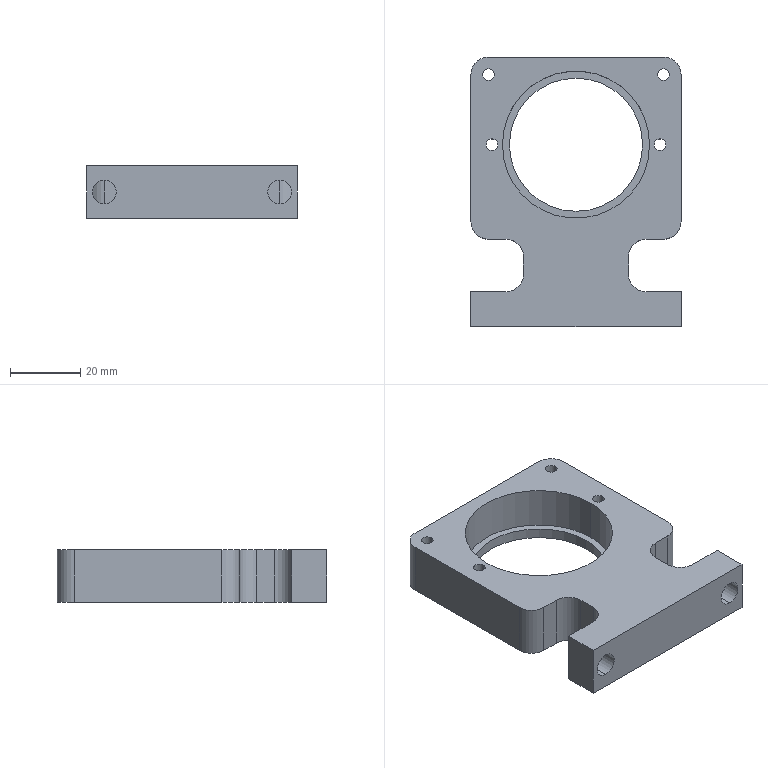Part | SolidWorks | features ICE 3, HoleWzd 2, Extrusion 1, Fillet 1 | 1 solid | 39 faces | box 60 x 77 x 15 mm | volume 41283 mm3 | cylinder 24 | plane 15 | commonest cylinder face diameters 3.3 x8 10 x8 6.8 x4 38 x2 42 x2
STEP:
#1=CARTESIAN_POINT('',(-26.65,72.,-7.5));
#2=VERTEX_POINT('',#1);
#3=CARTESIAN_POINT('',(-23.35,72.,-7.5));
#4=VERTEX_POINT('',#3);
#5=CARTESIAN_POINT('',(-25.,72.,-7.5));
#6=DIRECTION('',(0.,0.,1.));
#7=DIRECTION('',(1.,0.,0.));
#8=AXIS2_PLACEMENT_3D('',#5,#6,#7);
#9=CIRCLE('',#8,1.65);
#10=EDGE_CURVE('',#2,#4,#9,.T.);
#11=ORIENTED_EDGE('',*,*,#10,.F.);
#12=CARTESIAN_POINT('',(-26.65,72.,7.5));
#13=VERTEX_POINT('',#12);
#14=CARTESIAN_POINT('',(-26.65,72.,7.5));
#15=DIRECTION('',(0.,0.,1.));
#16=VECTOR('',#15,1000.);
#17=LINE('',#14,#16);
#18=EDGE_CURVE('',#2,#13,#17,.T.);
#19=ORIENTED_EDGE('',*,*,#18,.T.);
#20=CARTESIAN_POINT('',(-23.35,72.,7.5));
#21=VERTEX_POINT('',#20);
#22=CARTESIAN_POINT('',(-25.,72.,7.5));
#23=DIRECTION('',(0.,0.,1.));
#24=DIRECTION('',(1.,0.,0.));
#25=AXIS2_PLACEMENT_3D('',#22,#23,#24);
#26=CIRCLE('',#25,1.65);
#27=EDGE_CURVE('',#13,#21,#26,.T.);
#28=ORIENTED_EDGE('',*,*,#27,.T.);
#29=CARTESIAN_POINT('',(-23.35,72.,7.5));
#30=DIRECTION('',(0.,0.,1.));
#31=VECTOR('',#30,1000.);
#32=LINE('',#29,#31);
#33=EDGE_CURVE('',#4,#21,#32,.T.);
#34=ORIENTED_EDGE('',*,*,#33,.F.);
#35=EDGE_LOOP('',(#11,#19,#28,#34));
#36=FACE_OUTER_BOUND('',#35,.T.);
#37=CARTESIAN_POINT('',(-25.,72.,7.5));
#38=DIRECTION('',(0.,0.,1.));
#39=DIRECTION('',(1.,0.,0.));
#40=AXIS2_PLACEMENT_3D('',#37,#38,#39);
#41=CYLINDRICAL_SURFACE('',#40,1.65);
#42=ADVANCED_FACE('',(#36),#41,.F.);
#43=CARTESIAN_POINT('',(23.35,72.,-7.5));
#44=VERTEX_POINT('',#43);
#45=CARTESIAN_POINT('',(26.65,72.,-7.5));
#46=VERTEX_POINT('',#45);
#47=CARTESIAN_POINT('',(25.,72.,-7.5));
#48=DIRECTION('',(0.,0.,1.));
#49=DIRECTION('',(1.,0.,0.));
#50=AXIS2_PLACEMENT_3D('',#47,#48,#49);
#51=CIRCLE('',#50,1.65);
#52=EDGE_CURVE('',#44,#46,#51,.T.);
#53=ORIENTED_EDGE('',*,*,#52,.F.);
#54=CARTESIAN_POINT('',(23.35,72.,7.5));
#55=VERTEX_POINT('',#54);
#56=CARTESIAN_POINT('',(23.35,72.,7.5));
#57=DIRECTION('',(0.,0.,1.));
#58=VECTOR('',#57,1000.);
#59=LINE('',#56,#58);
#60=EDGE_CURVE('',#44,#55,#59,.T.);
#61=ORIENTED_EDGE('',*,*,#60,.T.);
#62=CARTESIAN_POINT('',(26.65,72.,7.5));
#63=VERTEX_POINT('',#62);
#64=CARTESIAN_POINT('',(25.,72.,7.5));
#65=DIRECTION('',(0.,0.,1.));
#66=DIRECTION('',(1.,0.,0.));
#67=AXIS2_PLACEMENT_3D('',#64,#65,#66);
#68=CIRCLE('',#67,1.65);
#69=EDGE_CURVE('',#55,#63,#68,.T.);
#70=ORIENTED_EDGE('',*,*,#69,.T.);
#71=CARTESIAN_POINT('',(26.65,72.,7.5));
#72=DIRECTION('',(0.,0.,1.));
#73=VECTOR('',#72,1000.);
#74=LINE('',#71,#73);
#75=EDGE_CURVE('',#46,#63,#74,.T.);
#76=ORIENTED_EDGE('',*,*,#75,.F.);
#77=EDGE_LOOP('',(#53,#61,#70,#76));
#78=FACE_OUTER_BOUND('',#77,.T.);
#79=CARTESIAN_POINT('',(25.,72.,7.5));
#80=DIRECTION('',(0.,0.,1.));
#81=DIRECTION('',(1.,0.,0.));
#82=AXIS2_PLACEMENT_3D('',#79,#80,#81);
#83=CYLINDRICAL_SURFACE('',#82,1.65);
#84=ADVANCED_FACE('',(#78),#83,.F.);
#85=CARTESIAN_POINT('',(22.35,52.,-7.5));
#86=VERTEX_POINT('',#85);
#87=CARTESIAN_POINT('',(25.65,52.,-7.5));
#88=VERTEX_POINT('',#87);
#89=CARTESIAN_POINT('',(24.,52.,-7.5));
#90=DIRECTION('',(0.,0.,1.));
#91=DIRECTION('',(1.,0.,0.));
#92=AXIS2_PLACEMENT_3D('',#89,#90,#91);
#93=CIRCLE('',#92,1.65);
#94=EDGE_CURVE('',#86,#88,#93,.T.);
#95=ORIENTED_EDGE('',*,*,#94,.F.);
#96=CARTESIAN_POINT('',(22.35,52.,7.5));
#97=VERTEX_POINT('',#96);
#98=CARTESIAN_POINT('',(22.35,52.,7.5));
#99=DIRECTION('',(0.,0.,1.));
#100=VECTOR('',#99,1000.);
#101=LINE('',#98,#100);
#102=EDGE_CURVE('',#86,#97,#101,.T.);
#103=ORIENTED_EDGE('',*,*,#102,.T.);
#104=CARTESIAN_POINT('',(25.65,52.,7.5));
#105=VERTEX_POINT('',#104);
#106=CARTESIAN_POINT('',(24.,52.,7.5));
#107=DIRECTION('',(0.,0.,1.));
#108=DIRECTION('',(1.,0.,0.));
#109=AXIS2_PLACEMENT_3D('',#106,#107,#108);
#110=CIRCLE('',#109,1.65);
#111=EDGE_CURVE('',#97,#105,#110,.T.);
#112=ORIENTED_EDGE('',*,*,#111,.T.);
#113=CARTESIAN_POINT('',(25.65,52.,7.5));
#114=DIRECTION('',(0.,0.,1.));
#115=VECTOR('',#114,1000.);
#116=LINE('',#113,#115);
#117=EDGE_CURVE('',#88,#105,#116,.T.);
#118=ORIENTED_EDGE('',*,*,#117,.F.);
#119=EDGE_LOOP('',(#95,#103,#112,#118));
#120=FACE_OUTER_BOUND('',#119,.T.);
#121=CARTESIAN_POINT('',(24.,52.,7.5));
#122=DIRECTION('',(0.,0.,1.));
#123=DIRECTION('',(1.,0.,0.));
#124=AXIS2_PLACEMENT_3D('',#121,#122,#123);
#125=CYLINDRICAL_SURFACE('',#124,1.65);
#126=ADVANCED_FACE('',(#120),#125,.F.);
#127=CARTESIAN_POINT('',(-25.65,52.,-7.5));
#128=VERTEX_POINT('',#127);
#129=CARTESIAN_POINT('',(-22.35,52.,-7.5));
#130=VERTEX_POINT('',#129);
#131=CARTESIAN_POINT('',(-24.,52.,-7.5));
#132=DIRECTION('',(0.,0.,1.));
#133=DIRECTION('',(1.,0.,0.));
#134=AXIS2_PLACEMENT_3D('',#131,#132,#133);
#135=CIRCLE('',#134,1.65);
#136=EDGE_CURVE('',#128,#130,#135,.T.);
#137=ORIENTED_EDGE('',*,*,#136,.F.);
#138=CARTESIAN_POINT('',(-25.65,52.,7.5));
#139=VERTEX_POINT('',#138);
#140=CARTESIAN_POINT('',(-25.65,52.,7.5));
#141=DIRECTION('',(0.,0.,1.));
#142=VECTOR('',#141,1000.);
#143=LINE('',#140,#142);
#144=EDGE_CURVE('',#128,#139,#143,.T.);
#145=ORIENTED_EDGE('',*,*,#144,.T.);
#146=CARTESIAN_POINT('',(-22.35,52.,7.5));
#147=VERTEX_POINT('',#146);
#148=CARTESIAN_POINT('',(-24.,52.,7.5));
#149=DIRECTION('',(0.,0.,1.));
#150=DIRECTION('',(1.,0.,0.));
#151=AXIS2_PLACEMENT_3D('',#148,#149,#150);
#152=CIRCLE('',#151,1.65);
#153=EDGE_CURVE('',#139,#147,#152,.T.);
#154=ORIENTED_EDGE('',*,*,#153,.T.);
#155=CARTESIAN_POINT('',(-22.35,52.,7.5));
#156=DIRECTION('',(0.,0.,1.));
#157=VECTOR('',#156,1000.);
#158=LINE('',#155,#157);
#159=EDGE_CURVE('',#130,#147,#158,.T.);
#160=ORIENTED_EDGE('',*,*,#159,.F.);
#161=EDGE_LOOP('',(#137,#145,#154,#160));
#162=FACE_OUTER_BOUND('',#161,.T.);
#163=CARTESIAN_POINT('',(-24.,52.,7.5));
#164=DIRECTION('',(0.,0.,1.));
#165=DIRECTION('',(1.,0.,0.));
#166=AXIS2_PLACEMENT_3D('',#163,#164,#165);
#167=CYLINDRICAL_SURFACE('',#166,1.65);
#168=ADVANCED_FACE('',(#162),#167,.F.);
#169=CARTESIAN_POINT('',(-21.,52.,-4.5));
#170=VERTEX_POINT('',#169);
#171=CARTESIAN_POINT('',(21.,52.,-4.5));
#172=VERTEX_POINT('',#171);
#173=CARTESIAN_POINT('',(0.,52.,-4.5));
#174=DIRECTION('',(0.,0.,1.));
#175=DIRECTION('',(1.,0.,0.));
#176=AXIS2_PLACEMENT_3D('',#173,#174,#175);
#177=CIRCLE('',#176,21.);
#178=EDGE_CURVE('',#170,#172,#177,.T.);
#179=ORIENTED_EDGE('',*,*,#178,.F.);
#180=CARTESIAN_POINT('',(-21.,52.,7.5));
#181=VERTEX_POINT('',#180);
#182=CARTESIAN_POINT('',(-21.,52.,-4.5));
#183=DIRECTION('',(0.,0.,1.));
#184=VECTOR('',#183,1000.);
#185=LINE('',#182,#184);
#186=EDGE_CURVE('',#170,#181,#185,.T.);
#187=ORIENTED_EDGE('',*,*,#186,.T.);
#188=CARTESIAN_POINT('',(21.,52.,7.5));
#189=VERTEX_POINT('',#188);
#190=CARTESIAN_POINT('',(0.,52.,7.5));
#191=DIRECTION('',(0.,0.,1.));
#192=DIRECTION('',(1.,0.,0.));
#193=AXIS2_PLACEMENT_3D('',#190,#191,#192);
#194=CIRCLE('',#193,21.);
#195=EDGE_CURVE('',#181,#189,#194,.T.);
#196=ORIENTED_EDGE('',*,*,#195,.T.);
#197=CARTESIAN_POINT('',(21.,52.,-4.5));
#198=DIRECTION('',(0.,0.,1.));
#199=VECTOR('',#198,1000.);
#200=LINE('',#197,#199);
#201=EDGE_CURVE('',#172,#189,#200,.T.);
#202=ORIENTED_EDGE('',*,*,#201,.F.);
#203=EDGE_LOOP('',(#179,#187,#196,#202));
#204=FACE_OUTER_BOUND('',#203,.T.);
#205=CARTESIAN_POINT('',(0.,52.,-4.5));
#206=DIRECTION('',(0.,0.,1.));
#207=DIRECTION('',(1.,0.,0.));
#208=AXIS2_PLACEMENT_3D('',#205,#206,#207);
#209=CYLINDRICAL_SURFACE('',#208,21.);
#210=ADVANCED_FACE('',(#204),#209,.F.);
#211=CARTESIAN_POINT('',(-25.,10.,3.4));
#212=VERTEX_POINT('',#211);
#213=CARTESIAN_POINT('',(-25.,10.,-3.4));
#214=VERTEX_POINT('',#213);
#215=CARTESIAN_POINT('',(-25.,10.,0.));
#216=DIRECTION('',(0.,-1.,0.));
#217=DIRECTION('',(0.,0.,-1.));
#218=AXIS2_PLACEMENT_3D('',#215,#216,#217);
#219=CIRCLE('',#218,3.4);
#220=EDGE_CURVE('',#212,#214,#219,.T.);
#221=ORIENTED_EDGE('',*,*,#220,.F.);
#222=CARTESIAN_POINT('',(-25.,0.,3.4));
#223=VERTEX_POINT('',#222);
#224=CARTESIAN_POINT('',(-25.,15.,3.4));
#225=DIRECTION('',(0.,-1.,0.));
#226=VECTOR('',#225,1000.);
#227=LINE('',#224,#226);
#228=EDGE_CURVE('',#212,#223,#227,.T.);
#229=ORIENTED_EDGE('',*,*,#228,.T.);
#230=CARTESIAN_POINT('',(-25.,0.,-3.4));
#231=VERTEX_POINT('',#230);
#232=CARTESIAN_POINT('',(-25.,0.,0.));
#233=DIRECTION('',(0.,-1.,0.));
#234=DIRECTION('',(0.,0.,-1.));
#235=AXIS2_PLACEMENT_3D('',#232,#233,#234);
#236=CIRCLE('',#235,3.4);
#237=EDGE_CURVE('',#223,#231,#236,.T.);
#238=ORIENTED_EDGE('',*,*,#237,.T.);
#239=CARTESIAN_POINT('',(-25.,15.,-3.4));
#240=DIRECTION('',(0.,-1.,0.));
#241=VECTOR('',#240,1000.);
#242=LINE('',#239,#241);
#243=EDGE_CURVE('',#214,#231,#242,.T.);
#244=ORIENTED_EDGE('',*,*,#243,.F.);
#245=EDGE_LOOP('',(#221,#229,#238,#244));
#246=FACE_OUTER_BOUND('',#245,.T.);
#247=CARTESIAN_POINT('',(-25.,15.,0.));
#248=DIRECTION('',(0.,-1.,0.));
#249=DIRECTION('',(0.,0.,-1.));
#250=AXIS2_PLACEMENT_3D('',#247,#248,#249);
#251=CYLINDRICAL_SURFACE('',#250,3.4);
#252=ADVANCED_FACE('',(#246),#251,.F.);
#253=CARTESIAN_POINT('',(25.,10.,3.4));
#254=VERTEX_POINT('',#253);
#255=CARTESIAN_POINT('',(25.,10.,-3.4));
#256=VERTEX_POINT('',#255);
#257=CARTESIAN_POINT('',(25.,10.,0.));
#258=DIRECTION('',(0.,-1.,0.));
#259=DIRECTION('',(0.,0.,-1.));
#260=AXIS2_PLACEMENT_3D('',#257,#258,#259);
#261=CIRCLE('',#260,3.4);
#262=EDGE_CURVE('',#254,#256,#261,.T.);
#263=ORIENTED_EDGE('',*,*,#262,.F.);
#264=CARTESIAN_POINT('',(25.,0.,3.4));
#265=VERTEX_POINT('',#264);
#266=CARTESIAN_POINT('',(25.,15.,3.4));
#267=DIRECTION('',(0.,-1.,0.));
#268=VECTOR('',#267,1000.);
#269=LINE('',#266,#268);
#270=EDGE_CURVE('',#254,#265,#269,.T.);
#271=ORIENTED_EDGE('',*,*,#270,.T.);
#272=CARTESIAN_POINT('',(25.,0.,-3.4));
#273=VERTEX_POINT('',#272);
#274=CARTESIAN_POINT('',(25.,0.,0.));
#275=DIRECTION('',(0.,-1.,0.));
#276=DIRECTION('',(0.,0.,1.));
#277=AXIS2_PLACEMENT_3D('',#274,#275,#276);
#278=CIRCLE('',#277,3.4);
#279=EDGE_CURVE('',#265,#273,#278,.T.);
#280=ORIENTED_EDGE('',*,*,#279,.T.);
#281=CARTESIAN_POINT('',(25.,15.,-3.4));
#282=DIRECTION('',(0.,-1.,0.));
#283=VECTOR('',#282,1000.);
#284=LINE('',#281,#283);
#285=EDGE_CURVE('',#256,#273,#284,.T.);
#286=ORIENTED_EDGE('',*,*,#285,.F.);
#287=EDGE_LOOP('',(#263,#271,#280,#286));
#288=FACE_OUTER_BOUND('',#287,.T.);
#289=CARTESIAN_POINT('',(25.,15.,0.));
#290=DIRECTION('',(0.,-1.,0.));
#291=DIRECTION('',(0.,0.,-1.));
#292=AXIS2_PLACEMENT_3D('',#289,#290,#291);
#293=CYLINDRICAL_SURFACE('',#292,3.4);
#294=ADVANCED_FACE('',(#288),#293,.F.);
#295=CARTESIAN_POINT('',(-19.,52.,-7.5));
#296=VERTEX_POINT('',#295);
#297=CARTESIAN_POINT('',(19.,52.,-7.5));
#298=VERTEX_POINT('',#297);
#299=CARTESIAN_POINT('',(0.,52.,-7.5));
#300=DIRECTION('',(0.,0.,1.));
#301=DIRECTION('',(1.,0.,0.));
#302=AXIS2_PLACEMENT_3D('',#299,#300,#301);
#303=CIRCLE('',#302,19.);
#304=EDGE_CURVE('',#296,#298,#303,.T.);
#305=ORIENTED_EDGE('',*,*,#304,.F.);
#306=CARTESIAN_POINT('',(-19.,52.,-4.5));
#307=VERTEX_POINT('',#306);
#308=CARTESIAN_POINT('',(-19.,52.,-7.5));
#309=DIRECTION('',(0.,0.,1.));
#310=VECTOR('',#309,1000.);
#311=LINE('',#308,#310);
#312=EDGE_CURVE('',#296,#307,#311,.T.);
#313=ORIENTED_EDGE('',*,*,#312,.T.);
#314=CARTESIAN_POINT('',(19.,52.,-4.5));
#315=VERTEX_POINT('',#314);
#316=CARTESIAN_POINT('',(0.,52.,-4.5));
#317=DIRECTION('',(0.,0.,-1.));
#318=DIRECTION('',(1.,0.,0.));
#319=AXIS2_PLACEMENT_3D('',#316,#317,#318);
#320=CIRCLE('',#319,19.);
#321=EDGE_CURVE('',#315,#307,#320,.T.);
#322=ORIENTED_EDGE('',*,*,#321,.F.);
#323=CARTESIAN_POINT('',(19.,52.,-7.5));
#324=DIRECTION('',(0.,0.,1.));
#325=VECTOR('',#324,1000.);
#326=LINE('',#323,#325);
#327=EDGE_CURVE('',#298,#315,#326,.T.);
#328=ORIENTED_EDGE('',*,*,#327,.F.);
#329=EDGE_LOOP('',(#305,#313,#322,#328));
#330=FACE_OUTER_BOUND('',#329,.T.);
#331=CARTESIAN_POINT('',(0.,52.,-7.5));
#332=DIRECTION('',(0.,0.,1.));
#333=DIRECTION('',(1.,0.,0.));
#334=AXIS2_PLACEMENT_3D('',#331,#332,#333);
#335=CYLINDRICAL_SURFACE('',#334,19.);
#336=ADVANCED_FACE('',(#330),#335,.F.);
#337=ORIENTED_EDGE('',*,*,#312,.F.);
#338=CARTESIAN_POINT('',(0.,52.,-7.5));
#339=DIRECTION('',(0.,0.,1.));
#340=DIRECTION('',(1.,0.,0.));
#341=AXIS2_PLACEMENT_3D('',#338,#339,#340);
#342=CIRCLE('',#341,19.);
#343=EDGE_CURVE('',#298,#296,#342,.T.);
#344=ORIENTED_EDGE('',*,*,#343,.F.);
#345=ORIENTED_EDGE('',*,*,#327,.T.);
#346=CARTESIAN_POINT('',(0.,52.,-4.5));
#347=DIRECTION('',(0.,0.,-1.));
#348=DIRECTION('',(1.,0.,0.));
#349=AXIS2_PLACEMENT_3D('',#346,#347,#348);
#350=CIRCLE('',#349,19.);
#351=EDGE_CURVE('',#307,#315,#350,.T.);
#352=ORIENTED_EDGE('',*,*,#351,.F.);
#353=EDGE_LOOP('',(#337,#344,#345,#352));
#354=FACE_OUTER_BOUND('',#353,.T.);
#355=CARTESIAN_POINT('',(0.,52.,-7.5));
#356=DIRECTION('',(0.,0.,1.));
#357=DIRECTION('',(1.,0.,0.));
#358=AXIS2_PLACEMENT_3D('',#355,#356,#357);
#359=CYLINDRICAL_SURFACE('',#358,19.);
#360=ADVANCED_FACE('',(#354),#359,.F.);
#361=CARTESIAN_POINT('',(-25.,25.,7.5));
#362=VERTEX_POINT('',#361);
#363=CARTESIAN_POINT('',(-20.,25.,7.5));
#364=VERTEX_POINT('',#363);
#365=CARTESIAN_POINT('',(-15.,25.,7.5));
#366=DIRECTION('',(1.,0.,0.));
#367=VECTOR('',#366,1000.);
#368=LINE('',#365,#367);
#369=EDGE_CURVE('',#362,#364,#368,.T.);
#370=ORIENTED_EDGE('',*,*,#369,.F.);
#371=CARTESIAN_POINT('',(-25.,25.,-7.5));
#372=VERTEX_POINT('',#371);
#373=CARTESIAN_POINT('',(-25.,25.,7.5));
#374=DIRECTION('',(0.,0.,-1.));
#375=VECTOR('',#374,1000.);
#376=LINE('',#373,#375);
#377=EDGE_CURVE('',#362,#372,#376,.T.);
#378=ORIENTED_EDGE('',*,*,#377,.T.);
#379=CARTESIAN_POINT('',(-20.,25.,-7.5));
#380=VERTEX_POINT('',#379);
#381=CARTESIAN_POINT('',(-15.,25.,-7.5));
#382=DIRECTION('',(1.,0.,0.));
#383=VECTOR('',#382,1000.);
#384=LINE('',#381,#383);
#385=EDGE_CURVE('',#372,#380,#384,.T.);
#386=ORIENTED_EDGE('',*,*,#385,.T.);
#387=CARTESIAN_POINT('',(-20.,25.,7.5));
#388=DIRECTION('',(0.,0.,1.));
#389=VECTOR('',#388,1000.);
#390=LINE('',#387,#389);
#391=EDGE_CURVE('',#380,#364,#390,.T.);
#392=ORIENTED_EDGE('',*,*,#391,.T.);
#393=EDGE_LOOP('',(#370,#378,#386,#392));
#394=FACE_OUTER_BOUND('',#393,.T.);
#395=CARTESIAN_POINT('',(-15.,25.,7.5));
#396=DIRECTION('',(0.,1.,0.));
#397=DIRECTION('',(-1.,0.,0.));
#398=AXIS2_PLACEMENT_3D('',#395,#396,#397);
#399=PLANE('',#398);
#400=ADVANCED_FACE('',(#394),#399,.F.);
#401=CARTESIAN_POINT('',(-15.,20.,-7.5));
#402=VERTEX_POINT('',#401);
#403=CARTESIAN_POINT('',(-15.,15.,-7.5));
#404=VERTEX_POINT('',#403);
#405=CARTESIAN_POINT('',(-15.,10.,-7.5));
#406=DIRECTION('',(0.,-1.,0.));
#407=VECTOR('',#406,1000.);
#408=LINE('',#405,#407);
#409=EDGE_CURVE('',#402,#404,#408,.T.);
#410=ORIENTED_EDGE('',*,*,#409,.T.);
#411=CARTESIAN_POINT('',(-15.,15.,7.5));
#412=VERTEX_POINT('',#411);
#413=CARTESIAN_POINT('',(-15.,15.,7.5));
#414=DIRECTION('',(0.,0.,1.));
#415=VECTOR('',#414,1000.);
#416=LINE('',#413,#415);
#417=EDGE_CURVE('',#404,#412,#416,.T.);
#418=ORIENTED_EDGE('',*,*,#417,.T.);
#419=CARTESIAN_POINT('',(-15.,20.,7.5));
#420=VERTEX_POINT('',#419);
#421=CARTESIAN_POINT('',(-15.,10.,7.5));
#422=DIRECTION('',(0.,-1.,0.));
#423=VECTOR('',#422,1000.);
#424=LINE('',#421,#423);
#425=EDGE_CURVE('',#420,#412,#424,.T.);
#426=ORIENTED_EDGE('',*,*,#425,.F.);
#427=CARTESIAN_POINT('',(-15.,20.,-7.5));
#428=DIRECTION('',(0.,0.,-1.));
#429=VECTOR('',#428,1000.);
#430=LINE('',#427,#429);
#431=EDGE_CURVE('',#420,#402,#430,.T.);
#432=ORIENTED_EDGE('',*,*,#431,.T.);
#433=EDGE_LOOP('',(#410,#418,#426,#432));
#434=FACE_OUTER_BOUND('',#433,.T.);
#435=CARTESIAN_POINT('',(-15.,10.,7.5));
#436=DIRECTION('',(1.,0.,0.));
#437=DIRECTION('',(0.,1.,0.));
#438=AXIS2_PLACEMENT_3D('',#435,#436,#437);
#439=PLANE('',#438);
#440=ADVANCED_FACE('',(#434),#439,.F.);
#441=CARTESIAN_POINT('',(-25.,10.,0.));
#442=DIRECTION('',(0.,-1.,0.));
#443=DIRECTION('',(0.,0.,-1.));
#444=AXIS2_PLACEMENT_3D('',#441,#442,#443);
#445=CIRCLE('',#444,3.4);
#446=EDGE_CURVE('',#214,#212,#445,.T.);
#447=ORIENTED_EDGE('',*,*,#446,.T.);
#448=ORIENTED_EDGE('',*,*,#220,.T.);
#449=EDGE_LOOP('',(#447,#448));
#450=FACE_BOUND('',#449,.T.);
#451=CARTESIAN_POINT('',(-20.,10.,7.5));
#452=VERTEX_POINT('',#451);
#453=CARTESIAN_POINT('',(-30.,10.,7.5));
#454=VERTEX_POINT('',#453);
#455=CARTESIAN_POINT('',(-30.,10.,7.5));
#456=DIRECTION('',(-1.,0.,0.));
#457=VECTOR('',#456,1000.);
#458=LINE('',#455,#457);
#459=EDGE_CURVE('',#452,#454,#458,.T.);
#460=ORIENTED_EDGE('',*,*,#459,.F.);
#461=CARTESIAN_POINT('',(-20.,10.,-7.5));
#462=VERTEX_POINT('',#461);
#463=CARTESIAN_POINT('',(-20.,10.,-7.5));
#464=DIRECTION('',(0.,0.,-1.));
#465=VECTOR('',#464,1000.);
#466=LINE('',#463,#465);
#467=EDGE_CURVE('',#452,#462,#466,.T.);
#468=ORIENTED_EDGE('',*,*,#467,.T.);
#469=CARTESIAN_POINT('',(-30.,10.,-7.5));
#470=VERTEX_POINT('',#469);
#471=CARTESIAN_POINT('',(-30.,10.,-7.5));
#472=DIRECTION('',(-1.,0.,0.));
#473=VECTOR('',#472,1000.);
#474=LINE('',#471,#473);
#475=EDGE_CURVE('',#462,#470,#474,.T.);
#476=ORIENTED_EDGE('',*,*,#475,.T.);
#477=CARTESIAN_POINT('',(-30.,10.,7.5));
#478=DIRECTION('',(0.,0.,-1.));
#479=VECTOR('',#478,1000.);
#480=LINE('',#477,#479);
#481=EDGE_CURVE('',#454,#470,#480,.T.);
#482=ORIENTED_EDGE('',*,*,#481,.F.);
#483=EDGE_LOOP('',(#460,#468,#476,#482));
#484=FACE_OUTER_BOUND('',#483,.T.);
#485=CARTESIAN_POINT('',(-30.,10.,7.5));
#486=DIRECTION('',(0.,-1.,0.));
#487=DIRECTION('',(0.,0.,-1.));
#488=AXIS2_PLACEMENT_3D('',#485,#486,#487);
#489=PLANE('',#488);
#490=ADVANCED_FACE('',(#450,#484),#489,.F.);
#491=CARTESIAN_POINT('',(-30.,0.,-7.5));
#492=VERTEX_POINT('',#491);
#493=CARTESIAN_POINT('',(-30.,0.,-7.5));
#494=DIRECTION('',(0.,-1.,0.));
#495=VECTOR('',#494,1000.);
#496=LINE('',#493,#495);
#497=EDGE_CURVE('',#470,#492,#496,.T.);
#498=ORIENTED_EDGE('',*,*,#497,.T.);
#499=CARTESIAN_POINT('',(-30.,0.,7.5));
#500=VERTEX_POINT('',#499);
#501=CARTESIAN_POINT('',(-30.,0.,7.5));
#502=DIRECTION('',(0.,0.,-1.));
#503=VECTOR('',#502,1000.);
#504=LINE('',#501,#503);
#505=EDGE_CURVE('',#500,#492,#504,.T.);
#506=ORIENTED_EDGE('',*,*,#505,.F.);
#507=CARTESIAN_POINT('',(-30.,0.,7.5));
#508=DIRECTION('',(0.,-1.,0.));
#509=VECTOR('',#508,1000.);
#510=LINE('',#507,#509);
#511=EDGE_CURVE('',#454,#500,#510,.T.);
#512=ORIENTED_EDGE('',*,*,#511,.F.);
#513=ORIENTED_EDGE('',*,*,#481,.T.);
#514=EDGE_LOOP('',(#498,#506,#512,#513));
#515=FACE_OUTER_BOUND('',#514,.T.);
#516=CARTESIAN_POINT('',(-30.,0.,7.5));
#517=DIRECTION('',(1.,0.,0.));
#518=DIRECTION('',(0.,0.,-1.));
#519=AXIS2_PLACEMENT_3D('',#516,#517,#518);
#520=PLANE('',#519);
#521=ADVANCED_FACE('',(#515),#520,.F.);
#522=CARTESIAN_POINT('',(-25.,0.,0.));
#523=DIRECTION('',(0.,-1.,0.));
#524=DIRECTION('',(0.,0.,-1.));
#525=AXIS2_PLACEMENT_3D('',#522,#523,#524);
#526=CIRCLE('',#525,3.4);
#527=EDGE_CURVE('',#231,#223,#526,.T.);
#528=ORIENTED_EDGE('',*,*,#527,.F.);
#529=ORIENTED_EDGE('',*,*,#237,.F.);
#530=EDGE_LOOP('',(#528,#529));
#531=FACE_BOUND('',#530,.T.);
#532=CARTESIAN_POINT('',(25.,0.,0.));
#533=DIRECTION('',(0.,-1.,0.));
#534=DIRECTION('',(0.,0.,1.));
#535=AXIS2_PLACEMENT_3D('',#532,#533,#534);
#536=CIRCLE('',#535,3.4);
#537=EDGE_CURVE('',#273,#265,#536,.T.);
#538=ORIENTED_EDGE('',*,*,#537,.F.);
#539=ORIENTED_EDGE('',*,*,#279,.F.);
#540=EDGE_LOOP('',(#538,#539));
#541=FACE_BOUND('',#540,.T.);
#542=CARTESIAN_POINT('',(30.,0.,-7.5));
#543=VERTEX_POINT('',#542);
#544=CARTESIAN_POINT('',(30.,0.,-7.5));
#545=DIRECTION('',(1.,0.,0.));
#546=VECTOR('',#545,1000.);
#547=LINE('',#544,#546);
#548=EDGE_CURVE('',#492,#543,#547,.T.);
#549=ORIENTED_EDGE('',*,*,#548,.T.);
#550=CARTESIAN_POINT('',(30.,0.,7.5));
#551=VERTEX_POINT('',#550);
#552=CARTESIAN_POINT('',(30.,0.,7.5));
#553=DIRECTION('',(0.,0.,-1.));
#554=VECTOR('',#553,1000.);
#555=LINE('',#552,#554);
#556=EDGE_CURVE('',#551,#543,#555,.T.);
#557=ORIENTED_EDGE('',*,*,#556,.F.);
#558=CARTESIAN_POINT('',(30.,0.,7.5));
#559=DIRECTION('',(1.,0.,0.));
#560=VECTOR('',#559,1000.);
#561=LINE('',#558,#560);
#562=EDGE_CURVE('',#500,#551,#561,.T.);
#563=ORIENTED_EDGE('',*,*,#562,.F.);
#564=ORIENTED_EDGE('',*,*,#505,.T.);
#565=EDGE_LOOP('',(#549,#557,#563,#564));
#566=FACE_OUTER_BOUND('',#565,.T.);
#567=CARTESIAN_POINT('',(30.,0.,7.5));
#568=DIRECTION('',(0.,1.,0.));
#569=DIRECTION('',(0.,0.,1.));
#570=AXIS2_PLACEMENT_3D('',#567,#568,#569);
#571=PLANE('',#570);
#572=ADVANCED_FACE('',(#531,#541,#566),#571,.F.);
#573=CARTESIAN_POINT('',(30.,10.,-7.5));
#574=VERTEX_POINT('',#573);
#575=CARTESIAN_POINT('',(30.,0.,-7.5));
#576=DIRECTION('',(0.,1.,0.));
#577=VECTOR('',#576,1000.);
#578=LINE('',#575,#577);
#579=EDGE_CURVE('',#543,#574,#578,.T.);
#580=ORIENTED_EDGE('',*,*,#579,.T.);
#581=CARTESIAN_POINT('',(30.,10.,7.5));
#582=VERTEX_POINT('',#581);
#583=CARTESIAN_POINT('',(30.,10.,7.5));
#584=DIRECTION('',(0.,0.,-1.));
#585=VECTOR('',#584,1000.);
#586=LINE('',#583,#585);
#587=EDGE_CURVE('',#582,#574,#586,.T.);
#588=ORIENTED_EDGE('',*,*,#587,.F.);
#589=CARTESIAN_POINT('',(30.,0.,7.5));
#590=DIRECTION('',(0.,1.,0.));
#591=VECTOR('',#590,1000.);
#592=LINE('',#589,#591);
#593=EDGE_CURVE('',#551,#582,#592,.T.);
#594=ORIENTED_EDGE('',*,*,#593,.F.);
#595=ORIENTED_EDGE('',*,*,#556,.T.);
#596=EDGE_LOOP('',(#580,#588,#594,#595));
#597=FACE_OUTER_BOUND('',#596,.T.);
#598=CARTESIAN_POINT('',(30.,0.,7.5));
#599=DIRECTION('',(-1.,0.,0.));
#600=DIRECTION('',(0.,0.,1.));
#601=AXIS2_PLACEMENT_3D('',#598,#599,#600);
#602=PLANE('',#601);
#603=ADVANCED_FACE('',(#597),#602,.F.);
#604=CARTESIAN_POINT('',(25.,10.,0.));
#605=DIRECTION('',(0.,-1.,0.));
#606=DIRECTION('',(0.,0.,-1.));
#607=AXIS2_PLACEMENT_3D('',#604,#605,#606);
#608=CIRCLE('',#607,3.4);
#609=EDGE_CURVE('',#256,#254,#608,.T.);
#610=ORIENTED_EDGE('',*,*,#609,.T.);
#611=ORIENTED_EDGE('',*,*,#262,.T.);
#612=EDGE_LOOP('',(#610,#611));
#613=FACE_BOUND('',#612,.T.);
#614=CARTESIAN_POINT('',(20.,10.,-7.5));
#615=VERTEX_POINT('',#614);
#616=CARTESIAN_POINT('',(30.,10.,-7.5));
#617=DIRECTION('',(-1.,0.,0.));
#618=VECTOR('',#617,1000.);
#619=LINE('',#616,#618);
#620=EDGE_CURVE('',#574,#615,#619,.T.);
#621=ORIENTED_EDGE('',*,*,#620,.T.);
#622=CARTESIAN_POINT('',(20.,10.,7.5));
#623=VERTEX_POINT('',#622);
#624=CARTESIAN_POINT('',(20.,10.,7.5));
#625=DIRECTION('',(0.,0.,1.));
#626=VECTOR('',#625,1000.);
#627=LINE('',#624,#626);
#628=EDGE_CURVE('',#615,#623,#627,.T.);
#629=ORIENTED_EDGE('',*,*,#628,.T.);
#630=CARTESIAN_POINT('',(30.,10.,7.5));
#631=DIRECTION('',(-1.,0.,0.));
#632=VECTOR('',#631,1000.);
#633=LINE('',#630,#632);
#634=EDGE_CURVE('',#582,#623,#633,.T.);
#635=ORIENTED_EDGE('',*,*,#634,.F.);
#636=ORIENTED_EDGE('',*,*,#587,.T.);
#637=EDGE_LOOP('',(#621,#629,#635,#636));
#638=FACE_OUTER_BOUND('',#637,.T.);
#639=CARTESIAN_POINT('',(30.,10.,7.5));
#640=DIRECTION('',(0.,-1.,0.));
#641=DIRECTION('',(0.,0.,-1.));
#642=AXIS2_PLACEMENT_3D('',#639,#640,#641);
#643=PLANE('',#642);
#644=ADVANCED_FACE('',(#613,#638),#643,.F.);
#645=CARTESIAN_POINT('',(15.,15.,-7.5));
#646=VERTEX_POINT('',#645);
#647=CARTESIAN_POINT('',(15.,20.,-7.5));
#648=VERTEX_POINT('',#647);
#649=CARTESIAN_POINT('',(15.,10.,-7.5));
#650=DIRECTION('',(0.,1.,0.));
#651=VECTOR('',#650,1000.);
#652=LINE('',#649,#651);
#653=EDGE_CURVE('',#646,#648,#652,.T.);
#654=ORIENTED_EDGE('',*,*,#653,.T.);
#655=CARTESIAN_POINT('',(15.,20.,7.5));
#656=VERTEX_POINT('',#655);
#657=CARTESIAN_POINT('',(15.,20.,7.5));
#658=DIRECTION('',(0.,0.,1.));
#659=VECTOR('',#658,1000.);
#660=LINE('',#657,#659);
#661=EDGE_CURVE('',#648,#656,#660,.T.);
#662=ORIENTED_EDGE('',*,*,#661,.T.);
#663=CARTESIAN_POINT('',(15.,15.,7.5));
#664=VERTEX_POINT('',#663);
#665=CARTESIAN_POINT('',(15.,10.,7.5));
#666=DIRECTION('',(0.,1.,0.));
#667=VECTOR('',#666,1000.);
#668=LINE('',#665,#667);
#669=EDGE_CURVE('',#664,#656,#668,.T.);
#670=ORIENTED_EDGE('',*,*,#669,.F.);
#671=CARTESIAN_POINT('',(15.,15.,-7.5));
#672=DIRECTION('',(0.,0.,-1.));
#673=VECTOR('',#672,1000.);
#674=LINE('',#671,#673);
#675=EDGE_CURVE('',#664,#646,#674,.T.);
#676=ORIENTED_EDGE('',*,*,#675,.T.);
#677=EDGE_LOOP('',(#654,#662,#670,#676));
#678=FACE_OUTER_BOUND('',#677,.T.);
#679=CARTESIAN_POINT('',(15.,10.,7.5));
#680=DIRECTION('',(-1.,0.,0.));
#681=DIRECTION('',(0.,-1.,0.));
#682=AXIS2_PLACEMENT_3D('',#679,#680,#681);
#683=PLANE('',#682);
#684=ADVANCED_FACE('',(#678),#683,.F.);
#685=CARTESIAN_POINT('',(20.,25.,-7.5));
#686=VERTEX_POINT('',#685);
#687=CARTESIAN_POINT('',(25.,25.,-7.5));
#688=VERTEX_POINT('',#687);
#689=CARTESIAN_POINT('',(15.,25.,-7.5));
#690=DIRECTION('',(1.,0.,0.));
#691=VECTOR('',#690,1000.);
#692=LINE('',#689,#691);
#693=EDGE_CURVE('',#686,#688,#692,.T.);
#694=ORIENTED_EDGE('',*,*,#693,.T.);
#695=CARTESIAN_POINT('',(25.,25.,7.5));
#696=VERTEX_POINT('',#695);
#697=CARTESIAN_POINT('',(25.,25.,7.5));
#698=DIRECTION('',(0.,0.,1.));
#699=VECTOR('',#698,1000.);
#700=LINE('',#697,#699);
#701=EDGE_CURVE('',#688,#696,#700,.T.);
#702=ORIENTED_EDGE('',*,*,#701,.T.);
#703=CARTESIAN_POINT('',(20.,25.,7.5));
#704=VERTEX_POINT('',#703);
#705=CARTESIAN_POINT('',(15.,25.,7.5));
#706=DIRECTION('',(1.,0.,0.));
#707=VECTOR('',#706,1000.);
#708=LINE('',#705,#707);
#709=EDGE_CURVE('',#704,#696,#708,.T.);
#710=ORIENTED_EDGE('',*,*,#709,.F.);
#711=CARTESIAN_POINT('',(20.,25.,-7.5));
#712=DIRECTION('',(0.,0.,-1.));
#713=VECTOR('',#712,1000.);
#714=LINE('',#711,#713);
#715=EDGE_CURVE('',#704,#686,#714,.T.);
#716=ORIENTED_EDGE('',*,*,#715,.T.);
#717=EDGE_LOOP('',(#694,#702,#710,#716));
#718=FACE_OUTER_BOUND('',#717,.T.);
#719=CARTESIAN_POINT('',(15.,25.,7.5));
#720=DIRECTION('',(0.,1.,0.));
#721=DIRECTION('',(-1.,0.,0.));
#722=AXIS2_PLACEMENT_3D('',#719,#720,#721);
#723=PLANE('',#722);
#724=ADVANCED_FACE('',(#718),#723,.F.);
#725=CARTESIAN_POINT('',(30.,30.,-7.5));
#726=VERTEX_POINT('',#725);
#727=CARTESIAN_POINT('',(30.,72.,-7.5));
#728=VERTEX_POINT('',#727);
#729=CARTESIAN_POINT('',(30.,25.,-7.5));
#730=DIRECTION('',(0.,1.,0.));
#731=VECTOR('',#730,1000.);
#732=LINE('',#729,#731);
#733=EDGE_CURVE('',#726,#728,#732,.T.);
#734=ORIENTED_EDGE('',*,*,#733,.T.);
#735=CARTESIAN_POINT('',(30.,72.,7.5));
#736=VERTEX_POINT('',#735);
#737=CARTESIAN_POINT('',(30.,72.,7.5));
#738=DIRECTION('',(0.,0.,1.));
#739=VECTOR('',#738,1000.);
#740=LINE('',#737,#739);
#741=EDGE_CURVE('',#728,#736,#740,.T.);
#742=ORIENTED_EDGE('',*,*,#741,.T.);
#743=CARTESIAN_POINT('',(30.,30.,7.5));
#744=VERTEX_POINT('',#743);
#745=CARTESIAN_POINT('',(30.,25.,7.5));
#746=DIRECTION('',(0.,1.,0.));
#747=VECTOR('',#746,1000.);
#748=LINE('',#745,#747);
#749=EDGE_CURVE('',#744,#736,#748,.T.);
#750=ORIENTED_EDGE('',*,*,#749,.F.);
#751=CARTESIAN_POINT('',(30.,30.,7.5));
#752=DIRECTION('',(0.,0.,-1.));
#753=VECTOR('',#752,1000.);
#754=LINE('',#751,#753);
#755=EDGE_CURVE('',#744,#726,#754,.T.);
#756=ORIENTED_EDGE('',*,*,#755,.T.);
#757=EDGE_LOOP('',(#734,#742,#750,#756));
#758=FACE_OUTER_BOUND('',#757,.T.);
#759=CARTESIAN_POINT('',(30.,25.,7.5));
#760=DIRECTION('',(-1.,0.,0.));
#761=DIRECTION('',(0.,0.,1.));
#762=AXIS2_PLACEMENT_3D('',#759,#760,#761);
#763=PLANE('',#762);
#764=ADVANCED_FACE('',(#758),#763,.F.);
#765=CARTESIAN_POINT('',(25.,77.,7.5));
#766=VERTEX_POINT('',#765);
#767=CARTESIAN_POINT('',(-25.,77.,7.5));
#768=VERTEX_POINT('',#767);
#769=CARTESIAN_POINT('',(-30.,77.,7.5));
#770=DIRECTION('',(-1.,0.,0.));
#771=VECTOR('',#770,1000.);
#772=LINE('',#769,#771);
#773=EDGE_CURVE('',#766,#768,#772,.T.);
#774=ORIENTED_EDGE('',*,*,#773,.F.);
#775=CARTESIAN_POINT('',(25.,77.,-7.5));
#776=VERTEX_POINT('',#775);
#777=CARTESIAN_POINT('',(25.,77.,7.5));
#778=DIRECTION('',(0.,0.,-1.));
#779=VECTOR('',#778,1000.);
#780=LINE('',#777,#779);
#781=EDGE_CURVE('',#766,#776,#780,.T.);
#782=ORIENTED_EDGE('',*,*,#781,.T.);
#783=CARTESIAN_POINT('',(-25.,77.,-7.5));
#784=VERTEX_POINT('',#783);
#785=CARTESIAN_POINT('',(-30.,77.,-7.5));
#786=DIRECTION('',(-1.,0.,0.));
#787=VECTOR('',#786,1000.);
#788=LINE('',#785,#787);
#789=EDGE_CURVE('',#776,#784,#788,.T.);
#790=ORIENTED_EDGE('',*,*,#789,.T.);
#791=CARTESIAN_POINT('',(-25.,77.,7.5));
#792=DIRECTION('',(0.,0.,1.));
#793=VECTOR('',#792,1000.);
#794=LINE('',#791,#793);
#795=EDGE_CURVE('',#784,#768,#794,.T.);
#796=ORIENTED_EDGE('',*,*,#795,.T.);
#797=EDGE_LOOP('',(#774,#782,#790,#796));
#798=FACE_OUTER_BOUND('',#797,.T.);
#799=CARTESIAN_POINT('',(-30.,77.,7.5));
#800=DIRECTION('',(0.,-1.,0.));
#801=DIRECTION('',(0.,0.,-1.));
#802=AXIS2_PLACEMENT_3D('',#799,#800,#801);
#803=PLANE('',#802);
#804=ADVANCED_FACE('',(#798),#803,.F.);
#805=CARTESIAN_POINT('',(-30.,72.,-7.5));
#806=VERTEX_POINT('',#805);
#807=CARTESIAN_POINT('',(-30.,30.,-7.5));
#808=VERTEX_POINT('',#807);
#809=CARTESIAN_POINT('',(-30.,25.,-7.5));
#810=DIRECTION('',(0.,-1.,0.));
#811=VECTOR('',#810,1000.);
#812=LINE('',#809,#811);
#813=EDGE_CURVE('',#806,#808,#812,.T.);
#814=ORIENTED_EDGE('',*,*,#813,.T.);
#815=CARTESIAN_POINT('',(-30.,30.,7.5));
#816=VERTEX_POINT('',#815);
#817=CARTESIAN_POINT('',(-30.,30.,7.5));
#818=DIRECTION('',(0.,0.,1.));
#819=VECTOR('',#818,1000.);
#820=LINE('',#817,#819);
#821=EDGE_CURVE('',#808,#816,#820,.T.);
#822=ORIENTED_EDGE('',*,*,#821,.T.);
#823=CARTESIAN_POINT('',(-30.,72.,7.5));
#824=VERTEX_POINT('',#823);
#825=CARTESIAN_POINT('',(-30.,25.,7.5));
#826=DIRECTION('',(0.,-1.,0.));
#827=VECTOR('',#826,1000.);
#828=LINE('',#825,#827);
#829=EDGE_CURVE('',#824,#816,#828,.T.);
#830=ORIENTED_EDGE('',*,*,#829,.F.);
#831=CARTESIAN_POINT('',(-30.,72.,7.5));
#832=DIRECTION('',(0.,0.,-1.));
#833=VECTOR('',#832,1000.);
#834=LINE('',#831,#833);
#835=EDGE_CURVE('',#824,#806,#834,.T.);
#836=ORIENTED_EDGE('',*,*,#835,.T.);
#837=EDGE_LOOP('',(#814,#822,#830,#836));
#838=FACE_OUTER_BOUND('',#837,.T.);
#839=CARTESIAN_POINT('',(-30.,25.,7.5));
#840=DIRECTION('',(1.,0.,0.));
#841=DIRECTION('',(0.,0.,-1.));
#842=AXIS2_PLACEMENT_3D('',#839,#840,#841);
#843=PLANE('',#842);
#844=ADVANCED_FACE('',(#838),#843,.F.);
#845=CARTESIAN_POINT('',(-25.,72.,7.5));
#846=DIRECTION('',(0.,0.,1.));
#847=DIRECTION('',(1.,0.,0.));
#848=AXIS2_PLACEMENT_3D('',#845,#846,#847);
#849=CIRCLE('',#848,1.65);
#850=EDGE_CURVE('',#21,#13,#849,.T.);
#851=ORIENTED_EDGE('',*,*,#850,.F.);
#852=ORIENTED_EDGE('',*,*,#27,.F.);
#853=EDGE_LOOP('',(#851,#852));
#854=FACE_BOUND('',#853,.T.);
#855=CARTESIAN_POINT('',(25.,72.,7.5));
#856=DIRECTION('',(0.,0.,1.));
#857=DIRECTION('',(1.,0.,0.));
#858=AXIS2_PLACEMENT_3D('',#855,#856,#857);
#859=CIRCLE('',#858,1.65);
#860=EDGE_CURVE('',#63,#55,#859,.T.);
#861=ORIENTED_EDGE('',*,*,#860,.F.);
#862=ORIENTED_EDGE('',*,*,#69,.F.);
#863=EDGE_LOOP('',(#861,#862));
#864=FACE_BOUND('',#863,.T.);
#865=CARTESIAN_POINT('',(24.,52.,7.5));
#866=DIRECTION('',(0.,0.,1.));
#867=DIRECTION('',(1.,0.,0.));
#868=AXIS2_PLACEMENT_3D('',#865,#866,#867);
#869=CIRCLE('',#868,1.65);
#870=EDGE_CURVE('',#105,#97,#869,.T.);
#871=ORIENTED_EDGE('',*,*,#870,.F.);
#872=ORIENTED_EDGE('',*,*,#111,.F.);
#873=EDGE_LOOP('',(#871,#872));
#874=FACE_BOUND('',#873,.T.);
#875=CARTESIAN_POINT('',(-24.,52.,7.5));
#876=DIRECTION('',(0.,0.,1.));
#877=DIRECTION('',(1.,0.,0.));
#878=AXIS2_PLACEMENT_3D('',#875,#876,#877);
#879=CIRCLE('',#878,1.65);
#880=EDGE_CURVE('',#147,#139,#879,.T.);
#881=ORIENTED_EDGE('',*,*,#880,.F.);
#882=ORIENTED_EDGE('',*,*,#153,.F.);
#883=EDGE_LOOP('',(#881,#882));
#884=FACE_BOUND('',#883,.T.);
#885=CARTESIAN_POINT('',(0.,52.,7.5));
#886=DIRECTION('',(0.,0.,1.));
#887=DIRECTION('',(1.,0.,0.));
#888=AXIS2_PLACEMENT_3D('',#885,#886,#887);
#889=CIRCLE('',#888,21.);
#890=EDGE_CURVE('',#189,#181,#889,.T.);
#891=ORIENTED_EDGE('',*,*,#890,.F.);
#892=ORIENTED_EDGE('',*,*,#195,.F.);
#893=EDGE_LOOP('',(#891,#892));
#894=FACE_BOUND('',#893,.T.);
#895=ORIENTED_EDGE('',*,*,#829,.T.);
#896=CARTESIAN_POINT('',(-25.,30.,7.5));
#897=DIRECTION('',(0.,0.,1.));
#898=DIRECTION('',(-1.,0.,0.));
#899=AXIS2_PLACEMENT_3D('',#896,#897,#898);
#900=CIRCLE('',#899,5.);
#901=EDGE_CURVE('',#816,#362,#900,.T.);
#902=ORIENTED_EDGE('',*,*,#901,.T.);
#903=ORIENTED_EDGE('',*,*,#369,.T.);
#904=CARTESIAN_POINT('',(-20.,20.,7.5));
#905=DIRECTION('',(0.,0.,-1.));
#906=DIRECTION('',(-1.,0.,0.));
#907=AXIS2_PLACEMENT_3D('',#904,#905,#906);
#908=CIRCLE('',#907,5.);
#909=EDGE_CURVE('',#364,#420,#908,.T.);
#910=ORIENTED_EDGE('',*,*,#909,.T.);
#911=ORIENTED_EDGE('',*,*,#425,.T.);
#912=CARTESIAN_POINT('',(-20.,15.,7.5));
#913=DIRECTION('',(0.,0.,-1.));
#914=DIRECTION('',(-1.,0.,0.));
#915=AXIS2_PLACEMENT_3D('',#912,#913,#914);
#916=CIRCLE('',#915,5.);
#917=EDGE_CURVE('',#412,#452,#916,.T.);
#918=ORIENTED_EDGE('',*,*,#917,.T.);
#919=ORIENTED_EDGE('',*,*,#459,.T.);
#920=ORIENTED_EDGE('',*,*,#511,.T.);
#921=ORIENTED_EDGE('',*,*,#562,.T.);
#922=ORIENTED_EDGE('',*,*,#593,.T.);
#923=ORIENTED_EDGE('',*,*,#634,.T.);
#924=CARTESIAN_POINT('',(20.,15.,7.5));
#925=DIRECTION('',(0.,0.,-1.));
#926=DIRECTION('',(-1.,0.,0.));
#927=AXIS2_PLACEMENT_3D('',#924,#925,#926);
#928=CIRCLE('',#927,5.);
#929=EDGE_CURVE('',#623,#664,#928,.T.);
#930=ORIENTED_EDGE('',*,*,#929,.T.);
#931=ORIENTED_EDGE('',*,*,#669,.T.);
#932=CARTESIAN_POINT('',(20.,20.,7.5));
#933=DIRECTION('',(0.,0.,-1.));
#934=DIRECTION('',(-1.,0.,0.));
#935=AXIS2_PLACEMENT_3D('',#932,#933,#934);
#936=CIRCLE('',#935,5.);
#937=EDGE_CURVE('',#656,#704,#936,.T.);
#938=ORIENTED_EDGE('',*,*,#937,.T.);
#939=ORIENTED_EDGE('',*,*,#709,.T.);
#940=CARTESIAN_POINT('',(25.,30.,7.5));
#941=DIRECTION('',(0.,0.,1.));
#942=DIRECTION('',(-1.,0.,0.));
#943=AXIS2_PLACEMENT_3D('',#940,#941,#942);
#944=CIRCLE('',#943,5.);
#945=EDGE_CURVE('',#696,#744,#944,.T.);
#946=ORIENTED_EDGE('',*,*,#945,.T.);
#947=ORIENTED_EDGE('',*,*,#749,.T.);
#948=CARTESIAN_POINT('',(25.,72.,7.5));
#949=DIRECTION('',(0.,0.,1.));
#950=DIRECTION('',(-1.,0.,0.));
#951=AXIS2_PLACEMENT_3D('',#948,#949,#950);
#952=CIRCLE('',#951,5.);
#953=EDGE_CURVE('',#736,#766,#952,.T.);
#954=ORIENTED_EDGE('',*,*,#953,.T.);
#955=ORIENTED_EDGE('',*,*,#773,.T.);
#956=CARTESIAN_POINT('',(-25.,72.,7.5));
#957=DIRECTION('',(0.,0.,1.));
#958=DIRECTION('',(-1.,0.,0.));
#959=AXIS2_PLACEMENT_3D('',#956,#957,#958);
#960=CIRCLE('',#959,5.);
#961=EDGE_CURVE('',#768,#824,#960,.T.);
#962=ORIENTED_EDGE('',*,*,#961,.T.);
#963=EDGE_LOOP('',(#895,#902,#903,#910,#911,#918,#919,#920,#921,#922,#923,#930,#931,#938,#939,#946,#947,#954,#955,#962));
#964=FACE_OUTER_BOUND('',#963,.T.);
#965=CARTESIAN_POINT('',(0.,0.,7.5));
#966=DIRECTION('',(0.,0.,-1.));
#967=DIRECTION('',(-1.,0.,0.));
#968=AXIS2_PLACEMENT_3D('',#965,#966,#967);
#969=PLANE('',#968);
#970=ADVANCED_FACE('',(#854,#864,#874,#884,#894,#964),#969,.F.);
#971=CARTESIAN_POINT('',(-25.,72.,-7.5));
#972=DIRECTION('',(0.,0.,1.));
#973=DIRECTION('',(1.,0.,0.));
#974=AXIS2_PLACEMENT_3D('',#971,#972,#973);
#975=CIRCLE('',#974,1.65);
#976=EDGE_CURVE('',#4,#2,#975,.T.);
#977=ORIENTED_EDGE('',*,*,#976,.T.);
#978=ORIENTED_EDGE('',*,*,#10,.T.);
#979=EDGE_LOOP('',(#977,#978));
#980=FACE_BOUND('',#979,.T.);
#981=CARTESIAN_POINT('',(25.,72.,-7.5));
#982=DIRECTION('',(0.,0.,1.));
#983=DIRECTION('',(1.,0.,0.));
#984=AXIS2_PLACEMENT_3D('',#981,#982,#983);
#985=CIRCLE('',#984,1.65);
#986=EDGE_CURVE('',#46,#44,#985,.T.);
#987=ORIENTED_EDGE('',*,*,#986,.T.);
#988=ORIENTED_EDGE('',*,*,#52,.T.);
#989=EDGE_LOOP('',(#987,#988));
#990=FACE_BOUND('',#989,.T.);
#991=CARTESIAN_POINT('',(24.,52.,-7.5));
#992=DIRECTION('',(0.,0.,1.));
#993=DIRECTION('',(1.,0.,0.));
#994=AXIS2_PLACEMENT_3D('',#991,#992,#993);
#995=CIRCLE('',#994,1.65);
#996=EDGE_CURVE('',#88,#86,#995,.T.);
#997=ORIENTED_EDGE('',*,*,#996,.T.);
#998=ORIENTED_EDGE('',*,*,#94,.T.);
#999=EDGE_LOOP('',(#997,#998));
#1000=FACE_BOUND('',#999,.T.);
#1001=CARTESIAN_POINT('',(-24.,52.,-7.5));
#1002=DIRECTION('',(0.,0.,1.));
#1003=DIRECTION('',(1.,0.,0.));
#1004=AXIS2_PLACEMENT_3D('',#1001,#1002,#1003);
#1005=CIRCLE('',#1004,1.65);
#1006=EDGE_CURVE('',#130,#128,#1005,.T.);
#1007=ORIENTED_EDGE('',*,*,#1006,.T.);
#1008=ORIENTED_EDGE('',*,*,#136,.T.);
#1009=EDGE_LOOP('',(#1007,#1008));
#1010=FACE_BOUND('',#1009,.T.);
#1011=ORIENTED_EDGE('',*,*,#343,.T.);
#1012=ORIENTED_EDGE('',*,*,#304,.T.);
#1013=EDGE_LOOP('',(#1011,#1012));
#1014=FACE_BOUND('',#1013,.T.);
#1015=ORIENTED_EDGE('',*,*,#385,.F.);
#1016=CARTESIAN_POINT('',(-25.,30.,-7.5));
#1017=DIRECTION('',(0.,0.,-1.));
#1018=DIRECTION('',(-1.,0.,0.));
#1019=AXIS2_PLACEMENT_3D('',#1016,#1017,#1018);
#1020=CIRCLE('',#1019,5.);
#1021=EDGE_CURVE('',#372,#808,#1020,.T.);
#1022=ORIENTED_EDGE('',*,*,#1021,.T.);
#1023=ORIENTED_EDGE('',*,*,#813,.F.);
#1024=CARTESIAN_POINT('',(-25.,72.,-7.5));
#1025=DIRECTION('',(0.,0.,-1.));
#1026=DIRECTION('',(-1.,0.,0.));
#1027=AXIS2_PLACEMENT_3D('',#1024,#1025,#1026);
#1028=CIRCLE('',#1027,5.);
#1029=EDGE_CURVE('',#806,#784,#1028,.T.);
#1030=ORIENTED_EDGE('',*,*,#1029,.T.);
#1031=ORIENTED_EDGE('',*,*,#789,.F.);
#1032=CARTESIAN_POINT('',(25.,72.,-7.5));
#1033=DIRECTION('',(0.,0.,-1.));
#1034=DIRECTION('',(-1.,0.,0.));
#1035=AXIS2_PLACEMENT_3D('',#1032,#1033,#1034);
#1036=CIRCLE('',#1035,5.);
#1037=EDGE_CURVE('',#776,#728,#1036,.T.);
#1038=ORIENTED_EDGE('',*,*,#1037,.T.);
#1039=ORIENTED_EDGE('',*,*,#733,.F.);
#1040=CARTESIAN_POINT('',(25.,30.,-7.5));
#1041=DIRECTION('',(0.,0.,-1.));
#1042=DIRECTION('',(-1.,0.,0.));
#1043=AXIS2_PLACEMENT_3D('',#1040,#1041,#1042);
#1044=CIRCLE('',#1043,5.);
#1045=EDGE_CURVE('',#726,#688,#1044,.T.);
#1046=ORIENTED_EDGE('',*,*,#1045,.T.);
#1047=ORIENTED_EDGE('',*,*,#693,.F.);
#1048=CARTESIAN_POINT('',(20.,20.,-7.5));
#1049=DIRECTION('',(0.,0.,1.));
#1050=DIRECTION('',(-1.,0.,0.));
#1051=AXIS2_PLACEMENT_3D('',#1048,#1049,#1050);
#1052=CIRCLE('',#1051,5.);
#1053=EDGE_CURVE('',#686,#648,#1052,.T.);
#1054=ORIENTED_EDGE('',*,*,#1053,.T.);
#1055=ORIENTED_EDGE('',*,*,#653,.F.);
#1056=CARTESIAN_POINT('',(20.,15.,-7.5));
#1057=DIRECTION('',(0.,0.,1.));
#1058=DIRECTION('',(-1.,0.,0.));
#1059=AXIS2_PLACEMENT_3D('',#1056,#1057,#1058);
#1060=CIRCLE('',#1059,5.);
#1061=EDGE_CURVE('',#646,#615,#1060,.T.);
#1062=ORIENTED_EDGE('',*,*,#1061,.T.);
#1063=ORIENTED_EDGE('',*,*,#620,.F.);
#1064=ORIENTED_EDGE('',*,*,#579,.F.);
#1065=ORIENTED_EDGE('',*,*,#548,.F.);
#1066=ORIENTED_EDGE('',*,*,#497,.F.);
#1067=ORIENTED_EDGE('',*,*,#475,.F.);
#1068=CARTESIAN_POINT('',(-20.,15.,-7.5));
#1069=DIRECTION('',(0.,0.,1.));
#1070=DIRECTION('',(-1.,0.,0.));
#1071=AXIS2_PLACEMENT_3D('',#1068,#1069,#1070);
#1072=CIRCLE('',#1071,5.);
#1073=EDGE_CURVE('',#462,#404,#1072,.T.);
#1074=ORIENTED_EDGE('',*,*,#1073,.T.);
#1075=ORIENTED_EDGE('',*,*,#409,.F.);
#1076=CARTESIAN_POINT('',(-20.,20.,-7.5));
#1077=DIRECTION('',(0.,0.,1.));
#1078=DIRECTION('',(-1.,0.,0.));
#1079=AXIS2_PLACEMENT_3D('',#1076,#1077,#1078);
#1080=CIRCLE('',#1079,5.);
#1081=EDGE_CURVE('',#402,#380,#1080,.T.);
#1082=ORIENTED_EDGE('',*,*,#1081,.T.);
#1083=EDGE_LOOP('',(#1015,#1022,#1023,#1030,#1031,#1038,#1039,#1046,#1047,#1054,#1055,#1062,#1063,#1064,#1065,#1066,#1067,#1074,#1075,#1082));
#1084=FACE_OUTER_BOUND('',#1083,.T.);
#1085=CARTESIAN_POINT('',(0.,0.,-7.5));
#1086=DIRECTION('',(0.,0.,-1.));
#1087=DIRECTION('',(-1.,0.,0.));
#1088=AXIS2_PLACEMENT_3D('',#1085,#1086,#1087);
#1089=PLANE('',#1088);
#1090=ADVANCED_FACE('',(#980,#990,#1000,#1010,#1014,#1084),#1089,.T.);
#1091=ORIENTED_EDGE('',*,*,#270,.F.);
#1092=ORIENTED_EDGE('',*,*,#609,.F.);
#1093=ORIENTED_EDGE('',*,*,#285,.T.);
#1094=ORIENTED_EDGE('',*,*,#537,.T.);
#1095=EDGE_LOOP('',(#1091,#1092,#1093,#1094));
#1096=FACE_OUTER_BOUND('',#1095,.T.);
#1097=CARTESIAN_POINT('',(25.,15.,0.));
#1098=DIRECTION('',(0.,-1.,0.));
#1099=DIRECTION('',(0.,0.,-1.));
#1100=AXIS2_PLACEMENT_3D('',#1097,#1098,#1099);
#1101=CYLINDRICAL_SURFACE('',#1100,3.4);
#1102=ADVANCED_FACE('',(#1096),#1101,.F.);
#1103=ORIENTED_EDGE('',*,*,#228,.F.);
#1104=ORIENTED_EDGE('',*,*,#446,.F.);
#1105=ORIENTED_EDGE('',*,*,#243,.T.);
#1106=ORIENTED_EDGE('',*,*,#527,.T.);
#1107=EDGE_LOOP('',(#1103,#1104,#1105,#1106));
#1108=FACE_OUTER_BOUND('',#1107,.T.);
#1109=CARTESIAN_POINT('',(-25.,15.,0.));
#1110=DIRECTION('',(0.,-1.,0.));
#1111=DIRECTION('',(0.,0.,-1.));
#1112=AXIS2_PLACEMENT_3D('',#1109,#1110,#1111);
#1113=CYLINDRICAL_SURFACE('',#1112,3.4);
#1114=ADVANCED_FACE('',(#1108),#1113,.F.);
#1115=CARTESIAN_POINT('',(0.,52.,-4.5));
#1116=DIRECTION('',(0.,0.,1.));
#1117=DIRECTION('',(1.,0.,0.));
#1118=AXIS2_PLACEMENT_3D('',#1115,#1116,#1117);
#1119=CIRCLE('',#1118,21.);
#1120=EDGE_CURVE('',#172,#170,#1119,.T.);
#1121=ORIENTED_EDGE('',*,*,#1120,.T.);
#1122=ORIENTED_EDGE('',*,*,#178,.T.);
#1123=EDGE_LOOP('',(#1121,#1122));
#1124=FACE_OUTER_BOUND('',#1123,.T.);
#1125=ORIENTED_EDGE('',*,*,#321,.T.);
#1126=ORIENTED_EDGE('',*,*,#351,.T.);
#1127=EDGE_LOOP('',(#1125,#1126));
#1128=FACE_BOUND('',#1127,.T.);
#1129=CARTESIAN_POINT('',(0.,52.,-4.5));
#1130=DIRECTION('',(0.,0.,1.));
#1131=DIRECTION('',(1.,0.,0.));
#1132=AXIS2_PLACEMENT_3D('',#1129,#1130,#1131);
#1133=PLANE('',#1132);
#1134=ADVANCED_FACE('',(#1124,#1128),#1133,.T.);
#1135=ORIENTED_EDGE('',*,*,#186,.F.);
#1136=ORIENTED_EDGE('',*,*,#1120,.F.);
#1137=ORIENTED_EDGE('',*,*,#201,.T.);
#1138=ORIENTED_EDGE('',*,*,#890,.T.);
#1139=EDGE_LOOP('',(#1135,#1136,#1137,#1138));
#1140=FACE_OUTER_BOUND('',#1139,.T.);
#1141=CARTESIAN_POINT('',(0.,52.,-4.5));
#1142=DIRECTION('',(0.,0.,1.));
#1143=DIRECTION('',(1.,0.,0.));
#1144=AXIS2_PLACEMENT_3D('',#1141,#1142,#1143);
#1145=CYLINDRICAL_SURFACE('',#1144,21.);
#1146=ADVANCED_FACE('',(#1140),#1145,.F.);
#1147=ORIENTED_EDGE('',*,*,#144,.F.);
#1148=ORIENTED_EDGE('',*,*,#1006,.F.);
#1149=ORIENTED_EDGE('',*,*,#159,.T.);
#1150=ORIENTED_EDGE('',*,*,#880,.T.);
#1151=EDGE_LOOP('',(#1147,#1148,#1149,#1150));
#1152=FACE_OUTER_BOUND('',#1151,.T.);
#1153=CARTESIAN_POINT('',(-24.,52.,7.5));
#1154=DIRECTION('',(0.,0.,1.));
#1155=DIRECTION('',(1.,0.,0.));
#1156=AXIS2_PLACEMENT_3D('',#1153,#1154,#1155);
#1157=CYLINDRICAL_SURFACE('',#1156,1.65);
#1158=ADVANCED_FACE('',(#1152),#1157,.F.);
#1159=ORIENTED_EDGE('',*,*,#102,.F.);
#1160=ORIENTED_EDGE('',*,*,#996,.F.);
#1161=ORIENTED_EDGE('',*,*,#117,.T.);
#1162=ORIENTED_EDGE('',*,*,#870,.T.);
#1163=EDGE_LOOP('',(#1159,#1160,#1161,#1162));
#1164=FACE_OUTER_BOUND('',#1163,.T.);
#1165=CARTESIAN_POINT('',(24.,52.,7.5));
#1166=DIRECTION('',(0.,0.,1.));
#1167=DIRECTION('',(1.,0.,0.));
#1168=AXIS2_PLACEMENT_3D('',#1165,#1166,#1167);
#1169=CYLINDRICAL_SURFACE('',#1168,1.65);
#1170=ADVANCED_FACE('',(#1164),#1169,.F.);
#1171=ORIENTED_EDGE('',*,*,#60,.F.);
#1172=ORIENTED_EDGE('',*,*,#986,.F.);
#1173=ORIENTED_EDGE('',*,*,#75,.T.);
#1174=ORIENTED_EDGE('',*,*,#860,.T.);
#1175=EDGE_LOOP('',(#1171,#1172,#1173,#1174));
#1176=FACE_OUTER_BOUND('',#1175,.T.);
#1177=CARTESIAN_POINT('',(25.,72.,7.5));
#1178=DIRECTION('',(0.,0.,1.));
#1179=DIRECTION('',(1.,0.,0.));
#1180=AXIS2_PLACEMENT_3D('',#1177,#1178,#1179);
#1181=CYLINDRICAL_SURFACE('',#1180,1.65);
#1182=ADVANCED_FACE('',(#1176),#1181,.F.);
#1183=ORIENTED_EDGE('',*,*,#18,.F.);
#1184=ORIENTED_EDGE('',*,*,#976,.F.);
#1185=ORIENTED_EDGE('',*,*,#33,.T.);
#1186=ORIENTED_EDGE('',*,*,#850,.T.);
#1187=EDGE_LOOP('',(#1183,#1184,#1185,#1186));
#1188=FACE_OUTER_BOUND('',#1187,.T.);
#1189=CARTESIAN_POINT('',(-25.,72.,7.5));
#1190=DIRECTION('',(0.,0.,1.));
#1191=DIRECTION('',(1.,0.,0.));
#1192=AXIS2_PLACEMENT_3D('',#1189,#1190,#1191);
#1193=CYLINDRICAL_SURFACE('',#1192,1.65);
#1194=ADVANCED_FACE('',(#1188),#1193,.F.);
#1195=ORIENTED_EDGE('',*,*,#901,.F.);
#1196=ORIENTED_EDGE('',*,*,#821,.F.);
#1197=ORIENTED_EDGE('',*,*,#1021,.F.);
#1198=ORIENTED_EDGE('',*,*,#377,.F.);
#1199=EDGE_LOOP('',(#1195,#1196,#1197,#1198));
#1200=FACE_OUTER_BOUND('',#1199,.T.);
#1201=CARTESIAN_POINT('',(-25.,30.,7.5));
#1202=DIRECTION('',(0.,0.,-1.));
#1203=DIRECTION('',(-1.,0.,0.));
#1204=AXIS2_PLACEMENT_3D('',#1201,#1202,#1203);
#1205=CYLINDRICAL_SURFACE('',#1204,5.);
#1206=ADVANCED_FACE('',(#1200),#1205,.T.);
#1207=ORIENTED_EDGE('',*,*,#953,.F.);
#1208=ORIENTED_EDGE('',*,*,#741,.F.);
#1209=ORIENTED_EDGE('',*,*,#1037,.F.);
#1210=ORIENTED_EDGE('',*,*,#781,.F.);
#1211=EDGE_LOOP('',(#1207,#1208,#1209,#1210));
#1212=FACE_OUTER_BOUND('',#1211,.T.);
#1213=CARTESIAN_POINT('',(25.,72.,7.5));
#1214=DIRECTION('',(0.,0.,-1.));
#1215=DIRECTION('',(-1.,0.,0.));
#1216=AXIS2_PLACEMENT_3D('',#1213,#1214,#1215);
#1217=CYLINDRICAL_SURFACE('',#1216,5.);
#1218=ADVANCED_FACE('',(#1212),#1217,.T.);
#1219=ORIENTED_EDGE('',*,*,#945,.F.);
#1220=ORIENTED_EDGE('',*,*,#701,.F.);
#1221=ORIENTED_EDGE('',*,*,#1045,.F.);
#1222=ORIENTED_EDGE('',*,*,#755,.F.);
#1223=EDGE_LOOP('',(#1219,#1220,#1221,#1222));
#1224=FACE_OUTER_BOUND('',#1223,.T.);
#1225=CARTESIAN_POINT('',(25.,30.,7.5));
#1226=DIRECTION('',(0.,0.,-1.));
#1227=DIRECTION('',(-1.,0.,0.));
#1228=AXIS2_PLACEMENT_3D('',#1225,#1226,#1227);
#1229=CYLINDRICAL_SURFACE('',#1228,5.);
#1230=ADVANCED_FACE('',(#1224),#1229,.T.);
#1231=ORIENTED_EDGE('',*,*,#937,.F.);
#1232=ORIENTED_EDGE('',*,*,#661,.F.);
#1233=ORIENTED_EDGE('',*,*,#1053,.F.);
#1234=ORIENTED_EDGE('',*,*,#715,.F.);
#1235=EDGE_LOOP('',(#1231,#1232,#1233,#1234));
#1236=FACE_OUTER_BOUND('',#1235,.T.);
#1237=CARTESIAN_POINT('',(20.,20.,7.5));
#1238=DIRECTION('',(0.,0.,1.));
#1239=DIRECTION('',(1.,0.,0.));
#1240=AXIS2_PLACEMENT_3D('',#1237,#1238,#1239);
#1241=CYLINDRICAL_SURFACE('',#1240,5.);
#1242=ADVANCED_FACE('',(#1236),#1241,.F.);
#1243=ORIENTED_EDGE('',*,*,#929,.F.);
#1244=ORIENTED_EDGE('',*,*,#628,.F.);
#1245=ORIENTED_EDGE('',*,*,#1061,.F.);
#1246=ORIENTED_EDGE('',*,*,#675,.F.);
#1247=EDGE_LOOP('',(#1243,#1244,#1245,#1246));
#1248=FACE_OUTER_BOUND('',#1247,.T.);
#1249=CARTESIAN_POINT('',(20.,15.,7.5));
#1250=DIRECTION('',(0.,0.,1.));
#1251=DIRECTION('',(1.,0.,0.));
#1252=AXIS2_PLACEMENT_3D('',#1249,#1250,#1251);
#1253=CYLINDRICAL_SURFACE('',#1252,5.);
#1254=ADVANCED_FACE('',(#1248),#1253,.F.);
#1255=ORIENTED_EDGE('',*,*,#917,.F.);
#1256=ORIENTED_EDGE('',*,*,#417,.F.);
#1257=ORIENTED_EDGE('',*,*,#1073,.F.);
#1258=ORIENTED_EDGE('',*,*,#467,.F.);
#1259=EDGE_LOOP('',(#1255,#1256,#1257,#1258));
#1260=FACE_OUTER_BOUND('',#1259,.T.);
#1261=CARTESIAN_POINT('',(-20.,15.,7.5));
#1262=DIRECTION('',(0.,0.,1.));
#1263=DIRECTION('',(1.,0.,0.));
#1264=AXIS2_PLACEMENT_3D('',#1261,#1262,#1263);
#1265=CYLINDRICAL_SURFACE('',#1264,5.);
#1266=ADVANCED_FACE('',(#1260),#1265,.F.);
#1267=ORIENTED_EDGE('',*,*,#909,.F.);
#1268=ORIENTED_EDGE('',*,*,#391,.F.);
#1269=ORIENTED_EDGE('',*,*,#1081,.F.);
#1270=ORIENTED_EDGE('',*,*,#431,.F.);
#1271=EDGE_LOOP('',(#1267,#1268,#1269,#1270));
#1272=FACE_OUTER_BOUND('',#1271,.T.);
#1273=CARTESIAN_POINT('',(-20.,20.,7.5));
#1274=DIRECTION('',(0.,0.,1.));
#1275=DIRECTION('',(1.,0.,0.));
#1276=AXIS2_PLACEMENT_3D('',#1273,#1274,#1275);
#1277=CYLINDRICAL_SURFACE('',#1276,5.);
#1278=ADVANCED_FACE('',(#1272),#1277,.F.);
#1279=ORIENTED_EDGE('',*,*,#961,.F.);
#1280=ORIENTED_EDGE('',*,*,#795,.F.);
#1281=ORIENTED_EDGE('',*,*,#1029,.F.);
#1282=ORIENTED_EDGE('',*,*,#835,.F.);
#1283=EDGE_LOOP('',(#1279,#1280,#1281,#1282));
#1284=FACE_OUTER_BOUND('',#1283,.T.);
#1285=CARTESIAN_POINT('',(-25.,72.,7.5));
#1286=DIRECTION('',(0.,0.,-1.));
#1287=DIRECTION('',(-1.,0.,0.));
#1288=AXIS2_PLACEMENT_3D('',#1285,#1286,#1287);
#1289=CYLINDRICAL_SURFACE('',#1288,5.);
#1290=ADVANCED_FACE('',(#1284),#1289,.T.);
#1291=CLOSED_SHELL('',(#42,#84,#126,#168,#210,#252,#294,#336,#360,#400,#440,#490,#521,#572,#603,#644,#684,#724,#764,#804,#844,#970,#1090,#1102,#1114,#1134,#1146,#1158,#1170,#1182,#1194,#1206,#1218,#1230,#1242,#1254,#1266,#1278,#1290));
#1292=MANIFOLD_SOLID_BREP('',#1291);
#1293=CARTESIAN_POINT('',(0.,0.,0.));
#1294=DIRECTION('',(0.,0.,1.));
#1295=DIRECTION('',(1.,0.,0.));
#1296=AXIS2_PLACEMENT_3D('',#1293,#1294,#1295);
#1297=(LENGTH_UNIT()NAMED_UNIT(*)SI_UNIT(.MILLI.,.METRE.));
#1298=UNCERTAINTY_MEASURE_WITH_UNIT(LENGTH_MEASURE(0.00001),#1297,'','');
#1299=(NAMED_UNIT(*)PLANE_ANGLE_UNIT()SI_UNIT($,.RADIAN.));
#1300=(NAMED_UNIT(*)SI_UNIT($,.STERADIAN.)SOLID_ANGLE_UNIT());
#1301=(GEOMETRIC_REPRESENTATION_CONTEXT(3)GLOBAL_UNCERTAINTY_ASSIGNED_CONTEXT((#1298))GLOBAL_UNIT_ASSIGNED_CONTEXT((#1297,#1299,#1300))REPRESENTATION_CONTEXT('',''));
#1302=ADVANCED_BREP_SHAPE_REPRESENTATION('',(#1292,#1296),#1301);